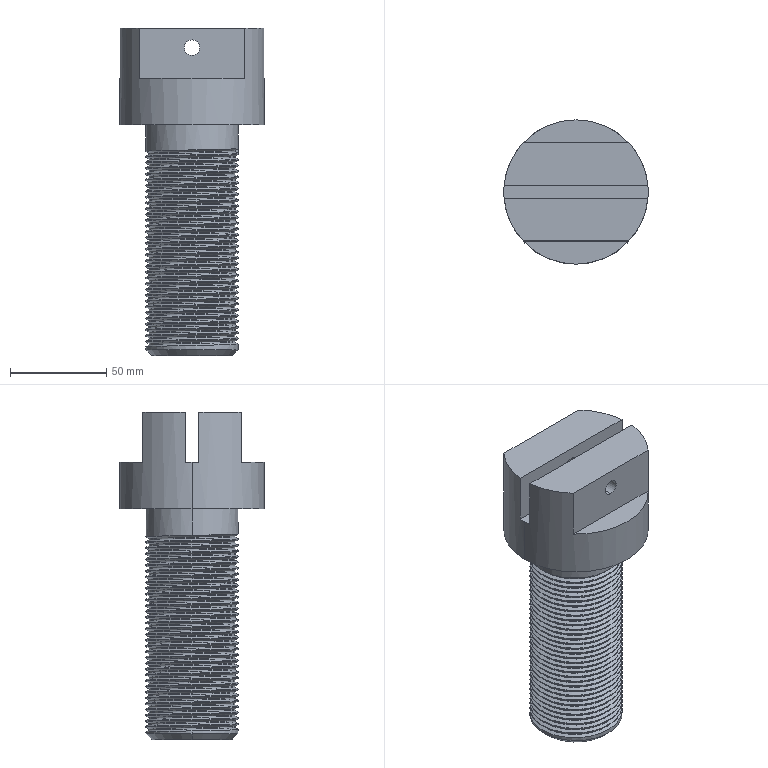Part | SolidWorks | features ICE 4, Chamfer 1, Extrusion 1, SweepThread 1 | 1 solid | 94 faces | box 75 x 75 x 170 mm | volume 384131 mm3 | cylinder 76 | plane 13 | spline 3 | cone 2 | commonest cylinder face diameters 48 x70 8 x4 75 x2